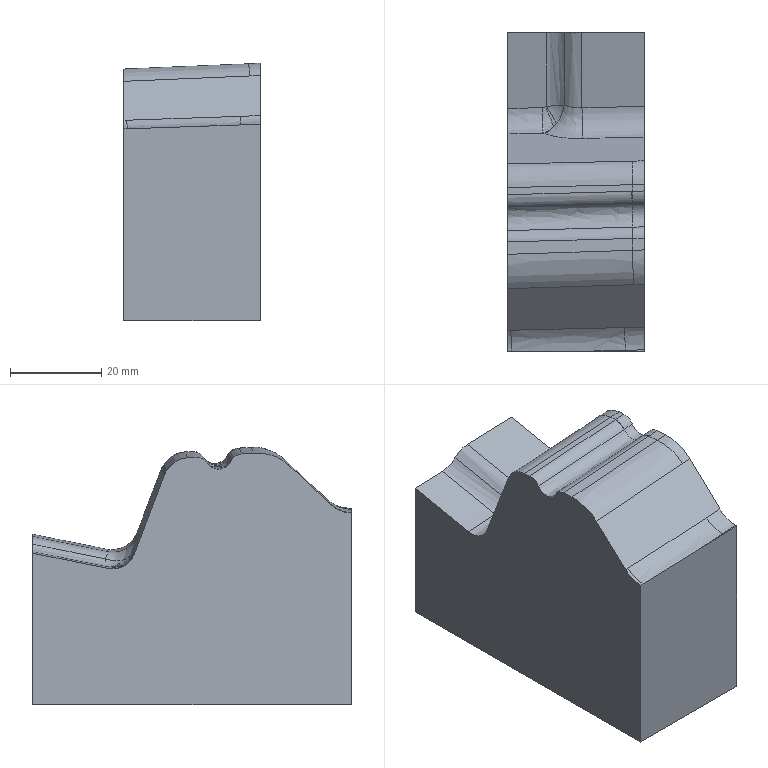Part | NX | features solid 2 | 1 solid | 39 faces | box 30 x 70.001 x 56.594 mm | volume 95080 mm3 | spline 34 | plane 5